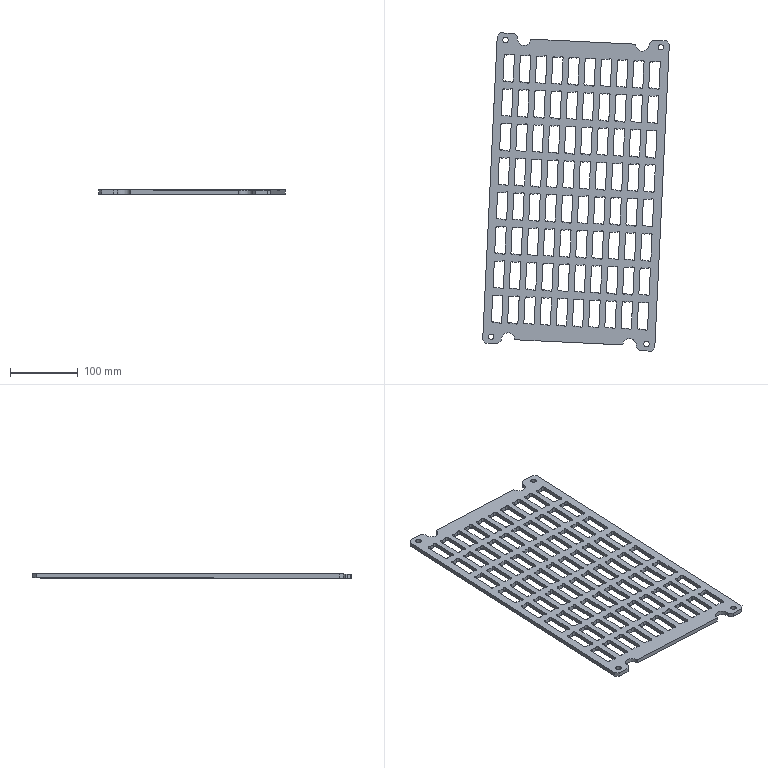Part | STEP file | X77-09401 | 1 solid | 758 faces | box 276.207 x 471.18 x 6.218 mm | volume 390241 mm3 | cylinder 414 | plane 184 | spline 160 | commonest cylinder face diameters 4 x400 8 x8 20 x6